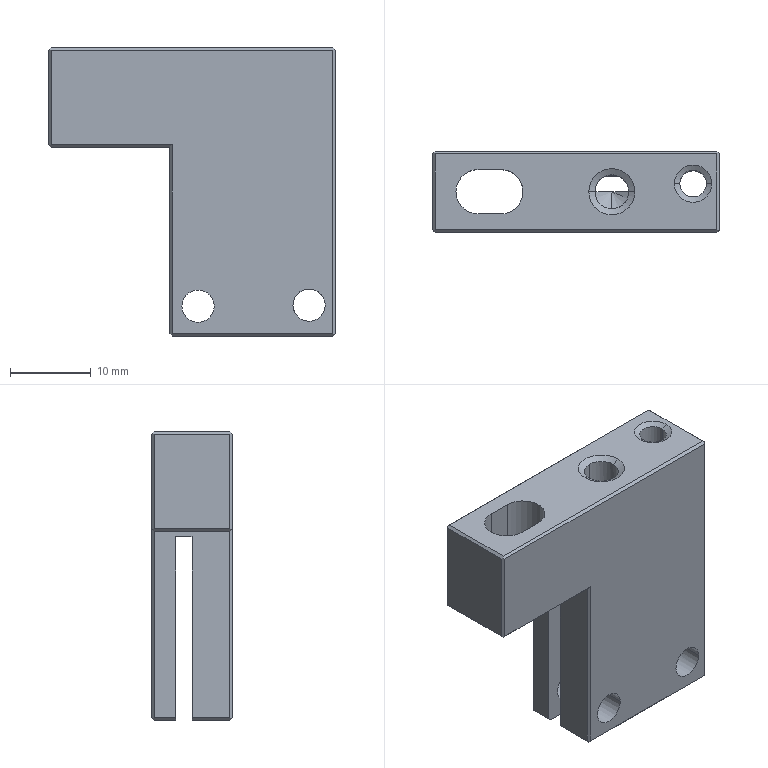Part | NX | 1 solid | 66 faces | box 35.5 x 10 x 35.7 mm | volume 7179 mm3 | plane 37 | cylinder 21 | cone 8 | commonest cylinder face diameters 4 x8 3.3 x6 4.2 x4 5.5 x3